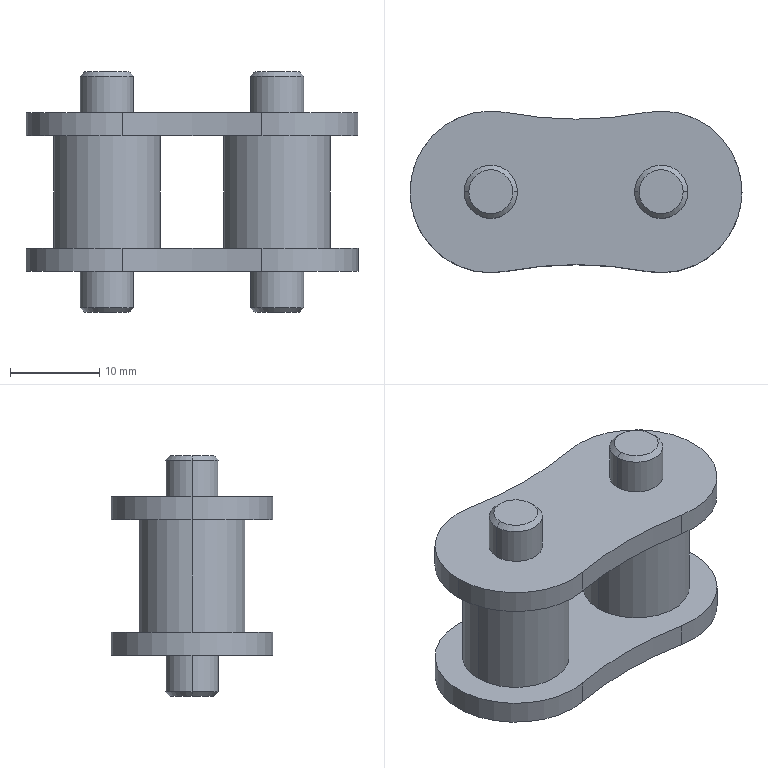Part | STEP file | 1 solid | 38 faces | box 37.13 x 18.08 x 26.9 mm | volume 6307 mm3 | cylinder 22 | cone 8 | plane 8 | commonest cylinder face diameters 5.96 x8 18.08 x6 11.91 x4 83.184 x4